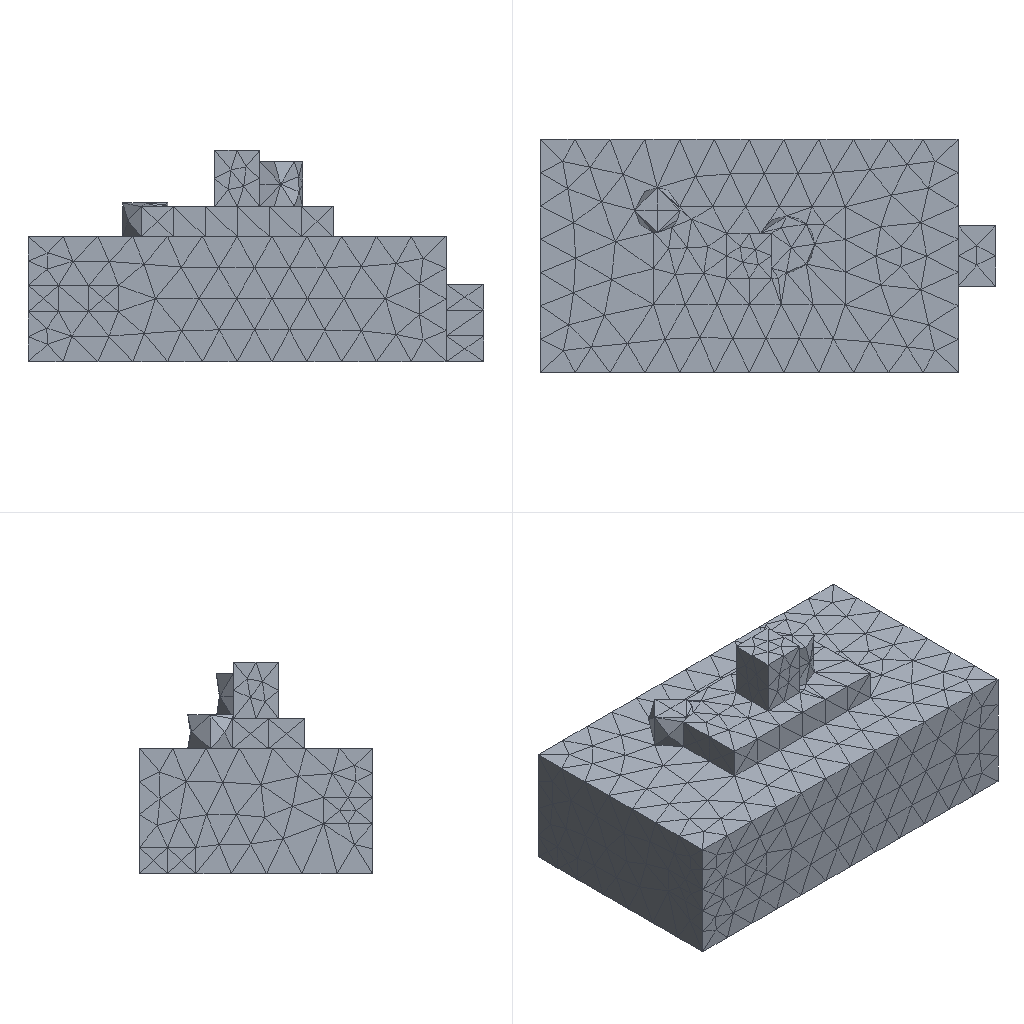Simulation study | ansys mapdl
Set-up summary:
category,name,step,type,value,unit,region
solver,ansys_mapdl
units,mm-N-s-tonne (MPa),,inferred,E=210000 density=
analysis,model,,static
mesh,nodes,,,5806
mesh,elements,,,3560
element_type,SOLID187,,,3560
material,mat 1,,E,210000
material,mat 1,,nu,0.3
load,,model,body load temp,,,all
load,,model,force,"1000 [dir=(0, 0, -1) n=317]",,node list
bc,,model,fixed,"[dofs=UX,UY,UZ n=6326]",,node list
Ansys APDL input file, long lists of numbers shortened:
/COM,ANSYS RELEASE 2026 R1           BUILD 26.1      UP20260202       09:08:28
/PREP7
/NOPR
/TITLE,2
ANTYPE, 0
*IF,_CDRDOFF,EQ,1,THEN     !if solid model was read in
_CDRDOFF=             !reset flag, numoffs already performed
*ELSE              !offset database for the following FE model
NUMOFF,NODE,     5806
NUMOFF,ELEM,     3560
NUMOFF,MAT ,        1
NUMOFF,TYPE,        1
*ENDIF
*SET,_RETURN ,  0.
*SET,_STATUS ,  0.
*SET,_UIQR   ,  317.
*SET,__FLOATPARAMETER__,  5806.
DOF,DELETE
ETBLOCK,        1,        1
(2i9,19a9)
        1      187        0        0        0        0        0        0        0        0        0        0        0        0        0        0        0        0        0        0        0
       -1
NBLOCK,6,SOLID,      5806,      5806
(3i9,6e21.13e3)
        1        0        0 6.0000000000000E+000 6.0000000000000E+000 5.6240000000000E+001
! (5805 more lines like these left out)
N,UNBL,LOC,       -1,
EBLOCK,19,SOLID,      3560,      3560
(19i10)
         1         1         1         1         0         0         0         0        10         0         1      2023      2024      2025      2026      2387      2388      2389      2390
! (7119 more lines like these left out)
        -1
MPTEMP,UNBL, 1, 1,  0.    ,
MPDATA,UNBL, 1,EX  ,       1, 1,  210000.000    ,
MPTEMP,UNBL, 1, 1,  0.    ,
MPDATA,UNBL, 1,NUXY,       1, 1, 0.3    ,
MPTEMP,UNBL, 1, 1,  0.    ,
MPDATA,UNBL, 1,PRXY,       1, 1, 0.3    ,
EXTOPT,ATTR,      0,      0,      0
EXTOPT,ESIZE,  0,  0.
EXTOPT,ACLEAR,      0
TREF,  0.
IRLF,  0
BFUNIF,TEMP,_TINY
ACEL,  0.    ,  0.    ,  0.
OMEGA,  0.    ,  0.    ,  0.
DOMEGA,  0.    ,  0.    ,  0.
CGLOC,  0.    ,  0.    ,  0.
CGOMEGA,  0.    ,  0.    ,  0.
DCGOMG,  0.    ,  0.    ,  0.
KUSE,     0
TIME,  0.
ALPHAD,  0.
BETAD,  0.
DMPRAT,  0.
DMPSTR,  0.
CRPLIM, 0.1    ,   0
CRPLIM,  0.    ,   1
NCNV,     0, 1.000000000E+12,     0,  0.    ,  0.
NEQIT,     0
ERESX,DEFA
DBLOCK,      6326
(i9,a6,2(pg16.9))
      332  UX    0.00000000      0.00000000
! (6325 more lines like these left out)
       -1
FBLOCK,       317
(i9,a6,2(pg16.9))
        1  FZ   -3.15457413      0.00000000
! (316 more lines like these left out)
       -1
/GO
FINISH
Results summary:
result,analysis_type_db,,,static,unstated
result,n_sets,,,1,unstated
result,load_steps[0].set,load_step=1,,1,unstated
result,load_steps[0].substep,load_step=1,,1,unstated
result,load_steps[0].time,load_step=1,,1,unstated
result,load_steps[0].freq,load_step=1,,1,unstated
result,load_steps[0].max_usum,load_step=1,,0.0005022,unstated
result,load_steps[0].max_seqv,load_step=1,,5.14,unstated
result,load_steps[0].reaction_sum.FX,load_step=1,,8.91613e-13,unstated
result,load_steps[0].reaction_sum.FY,load_step=1,,-7.61449e-12,unstated
result,load_steps[0].reaction_sum.FZ,load_step=1,,1000,unstated
result,load_steps[0].reaction_sum.MX,load_step=1,,0,unstated
result,load_steps[0].reaction_sum.MY,load_step=1,,0,unstated
result,load_steps[0].reaction_sum.MZ,load_step=1,,0,unstated
result,convergence,,,results present for all listed sets,unstated